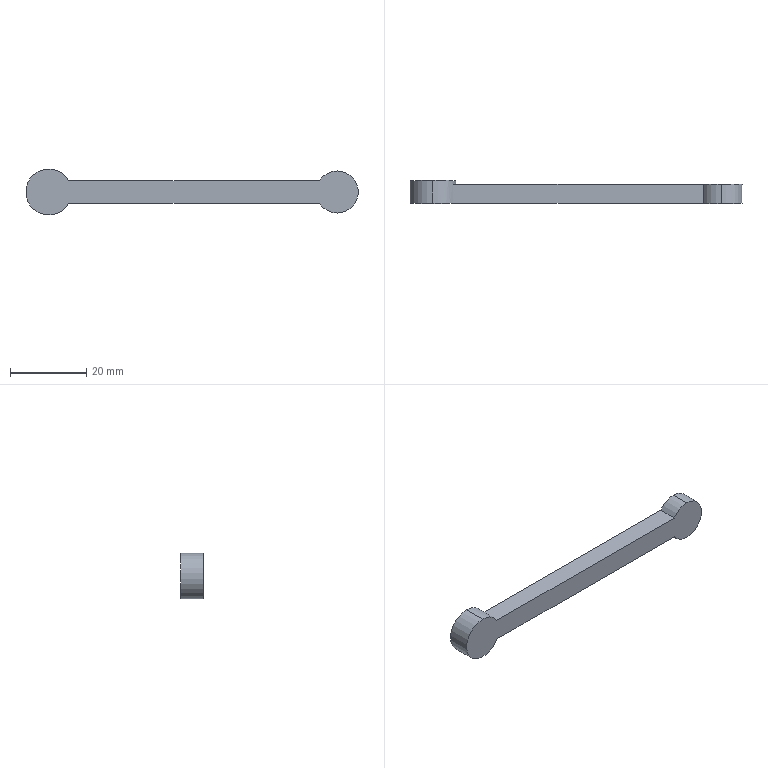Part | STEP file | 222_Default | 1 solid | 10 faces | box 86.9 x 6 x 12 mm | volume 3087 mm3 | cylinder 5 | plane 5 | commonest cylinder face diameters 11 x3 12 x2
STEP:
#1=CARTESIAN_POINT('',(0.,0.,0.));
#2=DIRECTION('',(0.,0.,1.));
#3=DIRECTION('',(1.,0.,0.));
#4=AXIS2_PLACEMENT_3D('',#1,#2,#3);
#5=CARTESIAN_POINT('',(37.7,0.,5.5));
#6=VERTEX_POINT('',#5);
#7=CARTESIAN_POINT('',(37.7,0.,-5.5));
#8=VERTEX_POINT('',#7);
#9=CARTESIAN_POINT('',(37.7,0.,0.));
#10=DIRECTION('',(0.,1.,0.));
#11=DIRECTION('',(0.,0.,1.));
#12=AXIS2_PLACEMENT_3D('',#9,#10,#11);
#13=CIRCLE('',#12,5.5);
#14=CARTESIAN_POINT('',(37.7,0.,0.));
#15=DIRECTION('',(0.,1.,0.));
#16=DIRECTION('',(0.,0.,1.));
#17=AXIS2_PLACEMENT_3D('',#14,#15,#16);
#18=CYLINDRICAL_SURFACE('',#17,5.5);
#19=CARTESIAN_POINT('',(0.,0.));
#20=DIRECTION('',(1.,0.));
#21=VECTOR('',#20,1.);
#22=LINE('',#19,#21);
#23=(GEOMETRIC_REPRESENTATION_CONTEXT(2)PARAMETRIC_REPRESENTATION_CONTEXT()REPRESENTATION_CONTEXT('',''));
#24=DEFINITIONAL_REPRESENTATION('',(#22),#23);
#25=PCURVE('',#18,#24);
#26=CARTESIAN_POINT('',(37.7,0.,0.));
#27=DIRECTION('',(0.,1.,0.));
#28=DIRECTION('',(0.,0.,1.));
#29=AXIS2_PLACEMENT_3D('',#26,#27,#28);
#30=PLANE('',#29);
#31=CARTESIAN_POINT('',(0.,0.));
#32=DIRECTION('',(1.,0.));
#33=AXIS2_PLACEMENT_2D('',#31,#32);
#34=CIRCLE('',#33,5.5);
#35=(GEOMETRIC_REPRESENTATION_CONTEXT(2)PARAMETRIC_REPRESENTATION_CONTEXT()REPRESENTATION_CONTEXT('',''));
#36=DEFINITIONAL_REPRESENTATION('',(#34),#35);
#37=PCURVE('',#30,#36);
#38=SURFACE_CURVE('',#13,(#25,#37),.PCURVE_S1.);
#39=EDGE_CURVE('',#6,#8,#38,.T.);
#40=ORIENTED_EDGE('',*,*,#39,.T.);
#41=CARTESIAN_POINT('',(37.7,5.,-5.5));
#42=VERTEX_POINT('',#41);
#43=CARTESIAN_POINT('',(37.7,0.,-5.5));
#44=DIRECTION('',(0.,1.,0.));
#45=VECTOR('',#44,1.);
#46=LINE('',#43,#45);
#47=CARTESIAN_POINT('',(3.142,0.));
#48=DIRECTION('',(0.,1.));
#49=VECTOR('',#48,1.);
#50=LINE('',#47,#49);
#51=(GEOMETRIC_REPRESENTATION_CONTEXT(2)PARAMETRIC_REPRESENTATION_CONTEXT()REPRESENTATION_CONTEXT('',''));
#52=DEFINITIONAL_REPRESENTATION('',(#50),#51);
#53=PCURVE('',#18,#52);
#54=CARTESIAN_POINT('',(37.7,0.,0.));
#55=DIRECTION('',(0.,1.,0.));
#56=DIRECTION('',(0.,0.,1.));
#57=AXIS2_PLACEMENT_3D('',#54,#55,#56);
#58=CYLINDRICAL_SURFACE('',#57,5.5);
#59=CARTESIAN_POINT('',(3.142,0.));
#60=DIRECTION('',(0.,1.));
#61=VECTOR('',#60,1.);
#62=LINE('',#59,#61);
#63=(GEOMETRIC_REPRESENTATION_CONTEXT(2)PARAMETRIC_REPRESENTATION_CONTEXT()REPRESENTATION_CONTEXT('',''));
#64=DEFINITIONAL_REPRESENTATION('',(#62),#63);
#65=PCURVE('',#58,#64);
#66=SURFACE_CURVE('',#46,(#53,#65),.PCURVE_S1.);
#67=EDGE_CURVE('',#8,#42,#66,.T.);
#68=ORIENTED_EDGE('',*,*,#67,.T.);
#69=CARTESIAN_POINT('',(37.7,5.,5.5));
#70=VERTEX_POINT('',#69);
#71=CARTESIAN_POINT('',(37.7,5.,0.));
#72=DIRECTION('',(0.,1.,0.));
#73=DIRECTION('',(0.,0.,1.));
#74=AXIS2_PLACEMENT_3D('',#71,#72,#73);
#75=CIRCLE('',#74,5.5);
#76=CARTESIAN_POINT('',(0.,5.));
#77=DIRECTION('',(1.,0.));
#78=VECTOR('',#77,1.);
#79=LINE('',#76,#78);
#80=(GEOMETRIC_REPRESENTATION_CONTEXT(2)PARAMETRIC_REPRESENTATION_CONTEXT()REPRESENTATION_CONTEXT('',''));
#81=DEFINITIONAL_REPRESENTATION('',(#79),#80);
#82=PCURVE('',#18,#81);
#83=CARTESIAN_POINT('',(37.7,5.,0.));
#84=DIRECTION('',(0.,1.,0.));
#85=DIRECTION('',(0.,0.,1.));
#86=AXIS2_PLACEMENT_3D('',#83,#84,#85);
#87=PLANE('',#86);
#88=CARTESIAN_POINT('',(0.,0.));
#89=DIRECTION('',(1.,0.));
#90=AXIS2_PLACEMENT_2D('',#88,#89);
#91=CIRCLE('',#90,5.5);
#92=(GEOMETRIC_REPRESENTATION_CONTEXT(2)PARAMETRIC_REPRESENTATION_CONTEXT()REPRESENTATION_CONTEXT('',''));
#93=DEFINITIONAL_REPRESENTATION('',(#91),#92);
#94=PCURVE('',#87,#93);
#95=SURFACE_CURVE('',#75,(#82,#94),.PCURVE_S1.);
#96=EDGE_CURVE('',#70,#42,#95,.T.);
#97=ORIENTED_EDGE('',*,*,#96,.F.);
#98=CARTESIAN_POINT('',(37.7,0.,5.5));
#99=DIRECTION('',(0.,1.,0.));
#100=VECTOR('',#99,1.);
#101=LINE('',#98,#100);
#102=CARTESIAN_POINT('',(0.,0.));
#103=DIRECTION('',(0.,1.));
#104=VECTOR('',#103,1.);
#105=LINE('',#102,#104);
#106=(GEOMETRIC_REPRESENTATION_CONTEXT(2)PARAMETRIC_REPRESENTATION_CONTEXT()REPRESENTATION_CONTEXT('',''));
#107=DEFINITIONAL_REPRESENTATION('',(#105),#106);
#108=PCURVE('',#18,#107);
#109=CARTESIAN_POINT('',(37.7,0.,0.));
#110=DIRECTION('',(0.,1.,0.));
#111=DIRECTION('',(0.,0.,1.));
#112=AXIS2_PLACEMENT_3D('',#109,#110,#111);
#113=CYLINDRICAL_SURFACE('',#112,5.5);
#114=CARTESIAN_POINT('',(6.283,0.));
#115=DIRECTION('',(0.,1.));
#116=VECTOR('',#115,1.);
#117=LINE('',#114,#116);
#118=(GEOMETRIC_REPRESENTATION_CONTEXT(2)PARAMETRIC_REPRESENTATION_CONTEXT()REPRESENTATION_CONTEXT('',''));
#119=DEFINITIONAL_REPRESENTATION('',(#117),#118);
#120=PCURVE('',#113,#119);
#121=SURFACE_CURVE('',#101,(#108,#120),.PCURVE_S1.);
#122=EDGE_CURVE('',#6,#70,#121,.T.);
#123=ORIENTED_EDGE('',*,*,#122,.F.);
#124=EDGE_LOOP('',(#40,#68,#97,#123));
#125=FACE_BOUND('',#124,.T.);
#126=ADVANCED_FACE('',(#125),#18,.T.);
#127=CARTESIAN_POINT('',(33.09,0.,3.));
#128=VERTEX_POINT('',#127);
#129=CARTESIAN_POINT('',(37.7,0.,0.));
#130=DIRECTION('',(0.,1.,0.));
#131=DIRECTION('',(0.,0.,1.));
#132=AXIS2_PLACEMENT_3D('',#129,#130,#131);
#133=CIRCLE('',#132,5.5);
#134=CARTESIAN_POINT('',(0.,0.));
#135=DIRECTION('',(1.,0.));
#136=VECTOR('',#135,1.);
#137=LINE('',#134,#136);
#138=(GEOMETRIC_REPRESENTATION_CONTEXT(2)PARAMETRIC_REPRESENTATION_CONTEXT()REPRESENTATION_CONTEXT('',''));
#139=DEFINITIONAL_REPRESENTATION('',(#137),#138);
#140=PCURVE('',#113,#139);
#141=CARTESIAN_POINT('',(0.,0.));
#142=DIRECTION('',(1.,0.));
#143=AXIS2_PLACEMENT_2D('',#141,#142);
#144=CIRCLE('',#143,5.5);
#145=(GEOMETRIC_REPRESENTATION_CONTEXT(2)PARAMETRIC_REPRESENTATION_CONTEXT()REPRESENTATION_CONTEXT('',''));
#146=DEFINITIONAL_REPRESENTATION('',(#144),#145);
#147=PCURVE('',#30,#146);
#148=SURFACE_CURVE('',#133,(#140,#147),.PCURVE_S1.);
#149=EDGE_CURVE('',#128,#6,#148,.T.);
#150=ORIENTED_EDGE('',*,*,#149,.T.);
#151=ORIENTED_EDGE('',*,*,#122,.T.);
#152=CARTESIAN_POINT('',(33.09,5.,3.));
#153=VERTEX_POINT('',#152);
#154=CARTESIAN_POINT('',(37.7,5.,0.));
#155=DIRECTION('',(0.,1.,0.));
#156=DIRECTION('',(0.,0.,1.));
#157=AXIS2_PLACEMENT_3D('',#154,#155,#156);
#158=CIRCLE('',#157,5.5);
#159=CARTESIAN_POINT('',(0.,5.));
#160=DIRECTION('',(1.,0.));
#161=VECTOR('',#160,1.);
#162=LINE('',#159,#161);
#163=(GEOMETRIC_REPRESENTATION_CONTEXT(2)PARAMETRIC_REPRESENTATION_CONTEXT()REPRESENTATION_CONTEXT('',''));
#164=DEFINITIONAL_REPRESENTATION('',(#162),#163);
#165=PCURVE('',#113,#164);
#166=CARTESIAN_POINT('',(0.,0.));
#167=DIRECTION('',(1.,0.));
#168=AXIS2_PLACEMENT_2D('',#166,#167);
#169=CIRCLE('',#168,5.5);
#170=(GEOMETRIC_REPRESENTATION_CONTEXT(2)PARAMETRIC_REPRESENTATION_CONTEXT()REPRESENTATION_CONTEXT('',''));
#171=DEFINITIONAL_REPRESENTATION('',(#169),#170);
#172=PCURVE('',#87,#171);
#173=SURFACE_CURVE('',#158,(#165,#172),.PCURVE_S1.);
#174=EDGE_CURVE('',#153,#70,#173,.T.);
#175=ORIENTED_EDGE('',*,*,#174,.F.);
#176=CARTESIAN_POINT('',(33.09,0.,3.));
#177=DIRECTION('',(0.,1.,0.));
#178=VECTOR('',#177,1.);
#179=LINE('',#176,#178);
#180=CARTESIAN_POINT('',(5.289,0.));
#181=DIRECTION('',(0.,1.));
#182=VECTOR('',#181,1.);
#183=LINE('',#180,#182);
#184=(GEOMETRIC_REPRESENTATION_CONTEXT(2)PARAMETRIC_REPRESENTATION_CONTEXT()REPRESENTATION_CONTEXT('',''));
#185=DEFINITIONAL_REPRESENTATION('',(#183),#184);
#186=PCURVE('',#113,#185);
#187=CARTESIAN_POINT('',(-32.504,0.,3.));
#188=DIRECTION('',(0.,0.,1.));
#189=DIRECTION('',(1.,0.,0.));
#190=AXIS2_PLACEMENT_3D('',#187,#188,#189);
#191=PLANE('',#190);
#192=CARTESIAN_POINT('',(65.594,0.));
#193=DIRECTION('',(0.,1.));
#194=VECTOR('',#193,1.);
#195=LINE('',#192,#194);
#196=(GEOMETRIC_REPRESENTATION_CONTEXT(2)PARAMETRIC_REPRESENTATION_CONTEXT()REPRESENTATION_CONTEXT('',''));
#197=DEFINITIONAL_REPRESENTATION('',(#195),#196);
#198=PCURVE('',#191,#197);
#199=SURFACE_CURVE('',#179,(#186,#198),.PCURVE_S1.);
#200=EDGE_CURVE('',#128,#153,#199,.T.);
#201=ORIENTED_EDGE('',*,*,#200,.F.);
#202=EDGE_LOOP('',(#150,#151,#175,#201));
#203=FACE_BOUND('',#202,.T.);
#204=ADVANCED_FACE('',(#203),#113,.T.);
#205=CARTESIAN_POINT('',(-37.7,6.,6.));
#206=VERTEX_POINT('',#205);
#207=CARTESIAN_POINT('',(-37.7,6.,-6.));
#208=VERTEX_POINT('',#207);
#209=CARTESIAN_POINT('',(-37.7,6.,0.));
#210=DIRECTION('',(0.,1.,0.));
#211=DIRECTION('',(0.,0.,1.));
#212=AXIS2_PLACEMENT_3D('',#209,#210,#211);
#213=CIRCLE('',#212,6.);
#214=CARTESIAN_POINT('',(-37.7,5.,0.));
#215=DIRECTION('',(0.,-1.,0.));
#216=DIRECTION('',(0.,0.,-1.));
#217=AXIS2_PLACEMENT_3D('',#214,#215,#216);
#218=CYLINDRICAL_SURFACE('',#217,6.);
#219=CARTESIAN_POINT('',(3.142,-1.));
#220=DIRECTION('',(-1.,0.));
#221=VECTOR('',#220,1.);
#222=LINE('',#219,#221);
#223=(GEOMETRIC_REPRESENTATION_CONTEXT(2)PARAMETRIC_REPRESENTATION_CONTEXT()REPRESENTATION_CONTEXT('',''));
#224=DEFINITIONAL_REPRESENTATION('',(#222),#223);
#225=PCURVE('',#218,#224);
#226=CARTESIAN_POINT('',(-37.7,6.,0.));
#227=DIRECTION('',(0.,1.,0.));
#228=DIRECTION('',(0.,0.,1.));
#229=AXIS2_PLACEMENT_3D('',#226,#227,#228);
#230=PLANE('',#229);
#231=CARTESIAN_POINT('',(0.,0.));
#232=DIRECTION('',(1.,0.));
#233=AXIS2_PLACEMENT_2D('',#231,#232);
#234=CIRCLE('',#233,6.);
#235=(GEOMETRIC_REPRESENTATION_CONTEXT(2)PARAMETRIC_REPRESENTATION_CONTEXT()REPRESENTATION_CONTEXT('',''));
#236=DEFINITIONAL_REPRESENTATION('',(#234),#235);
#237=PCURVE('',#230,#236);
#238=SURFACE_CURVE('',#213,(#225,#237),.PCURVE_S1.);
#239=EDGE_CURVE('',#206,#208,#238,.T.);
#240=ORIENTED_EDGE('',*,*,#239,.F.);
#241=CARTESIAN_POINT('',(-37.7,0.,6.));
#242=VERTEX_POINT('',#241);
#243=CARTESIAN_POINT('',(-37.7,5.,6.));
#244=DIRECTION('',(0.,-1.,0.));
#245=VECTOR('',#244,1.);
#246=LINE('',#243,#245);
#247=CARTESIAN_POINT('',(3.142,0.));
#248=DIRECTION('',(0.,1.));
#249=VECTOR('',#248,1.);
#250=LINE('',#247,#249);
#251=(GEOMETRIC_REPRESENTATION_CONTEXT(2)PARAMETRIC_REPRESENTATION_CONTEXT()REPRESENTATION_CONTEXT('',''));
#252=DEFINITIONAL_REPRESENTATION('',(#250),#251);
#253=PCURVE('',#218,#252);
#254=CARTESIAN_POINT('',(-37.7,5.,0.));
#255=DIRECTION('',(0.,-1.,0.));
#256=DIRECTION('',(0.,0.,-1.));
#257=AXIS2_PLACEMENT_3D('',#254,#255,#256);
#258=CYLINDRICAL_SURFACE('',#257,6.);
#259=CARTESIAN_POINT('',(3.142,0.));
#260=DIRECTION('',(0.,1.));
#261=VECTOR('',#260,1.);
#262=LINE('',#259,#261);
#263=(GEOMETRIC_REPRESENTATION_CONTEXT(2)PARAMETRIC_REPRESENTATION_CONTEXT()REPRESENTATION_CONTEXT('',''));
#264=DEFINITIONAL_REPRESENTATION('',(#262),#263);
#265=PCURVE('',#258,#264);
#266=SURFACE_CURVE('',#246,(#253,#265),.PCURVE_S1.);
#267=EDGE_CURVE('',#206,#242,#266,.T.);
#268=ORIENTED_EDGE('',*,*,#267,.T.);
#269=CARTESIAN_POINT('',(-32.504,0.,3.));
#270=VERTEX_POINT('',#269);
#271=CARTESIAN_POINT('',(-37.7,0.,0.));
#272=DIRECTION('',(0.,1.,0.));
#273=DIRECTION('',(0.,0.,1.));
#274=AXIS2_PLACEMENT_3D('',#271,#272,#273);
#275=CIRCLE('',#274,6.);
#276=CARTESIAN_POINT('',(3.142,5.));
#277=DIRECTION('',(-1.,0.));
#278=VECTOR('',#277,1.);
#279=LINE('',#276,#278);
#280=(GEOMETRIC_REPRESENTATION_CONTEXT(2)PARAMETRIC_REPRESENTATION_CONTEXT()REPRESENTATION_CONTEXT('',''));
#281=DEFINITIONAL_REPRESENTATION('',(#279),#280);
#282=PCURVE('',#218,#281);
#283=CARTESIAN_POINT('',(0.,-75.4));
#284=DIRECTION('',(1.,0.));
#285=AXIS2_PLACEMENT_2D('',#283,#284);
#286=CIRCLE('',#285,6.);
#287=(GEOMETRIC_REPRESENTATION_CONTEXT(2)PARAMETRIC_REPRESENTATION_CONTEXT()REPRESENTATION_CONTEXT('',''));
#288=DEFINITIONAL_REPRESENTATION('',(#286),#287);
#289=PCURVE('',#30,#288);
#290=SURFACE_CURVE('',#275,(#282,#289),.PCURVE_S1.);
#291=EDGE_CURVE('',#242,#270,#290,.T.);
#292=ORIENTED_EDGE('',*,*,#291,.T.);
#293=CARTESIAN_POINT('',(-32.504,5.,3.));
#294=VERTEX_POINT('',#293);
#295=CARTESIAN_POINT('',(-32.504,0.,3.));
#296=DIRECTION('',(0.,1.,0.));
#297=VECTOR('',#296,1.);
#298=LINE('',#295,#297);
#299=CARTESIAN_POINT('',(2.094,5.));
#300=DIRECTION('',(0.,-1.));
#301=VECTOR('',#300,1.);
#302=LINE('',#299,#301);
#303=(GEOMETRIC_REPRESENTATION_CONTEXT(2)PARAMETRIC_REPRESENTATION_CONTEXT()REPRESENTATION_CONTEXT('',''));
#304=DEFINITIONAL_REPRESENTATION('',(#302),#303);
#305=PCURVE('',#218,#304);
#306=CARTESIAN_POINT('',(0.,0.));
#307=DIRECTION('',(0.,1.));
#308=VECTOR('',#307,1.);
#309=LINE('',#306,#308);
#310=(GEOMETRIC_REPRESENTATION_CONTEXT(2)PARAMETRIC_REPRESENTATION_CONTEXT()REPRESENTATION_CONTEXT('',''));
#311=DEFINITIONAL_REPRESENTATION('',(#309),#310);
#312=PCURVE('',#191,#311);
#313=SURFACE_CURVE('',#298,(#305,#312),.PCURVE_S1.);
#314=EDGE_CURVE('',#270,#294,#313,.T.);
#315=ORIENTED_EDGE('',*,*,#314,.T.);
#316=CARTESIAN_POINT('',(-32.504,5.,-3.));
#317=VERTEX_POINT('',#316);
#318=CARTESIAN_POINT('',(-37.7,5.,0.));
#319=DIRECTION('',(0.,1.,0.));
#320=DIRECTION('',(0.,0.,1.));
#321=AXIS2_PLACEMENT_3D('',#318,#319,#320);
#322=CIRCLE('',#321,6.);
#323=CARTESIAN_POINT('',(3.142,0.));
#324=DIRECTION('',(-1.,0.));
#325=VECTOR('',#324,1.);
#326=LINE('',#323,#325);
#327=(GEOMETRIC_REPRESENTATION_CONTEXT(2)PARAMETRIC_REPRESENTATION_CONTEXT()REPRESENTATION_CONTEXT('',''));
#328=DEFINITIONAL_REPRESENTATION('',(#326),#327);
#329=PCURVE('',#218,#328);
#330=CARTESIAN_POINT('',(0.,-75.4));
#331=DIRECTION('',(1.,0.));
#332=AXIS2_PLACEMENT_2D('',#330,#331);
#333=CIRCLE('',#332,6.);
#334=(GEOMETRIC_REPRESENTATION_CONTEXT(2)PARAMETRIC_REPRESENTATION_CONTEXT()REPRESENTATION_CONTEXT('',''));
#335=DEFINITIONAL_REPRESENTATION('',(#333),#334);
#336=PCURVE('',#87,#335);
#337=SURFACE_CURVE('',#322,(#329,#336),.PCURVE_S1.);
#338=EDGE_CURVE('',#294,#317,#337,.T.);
#339=ORIENTED_EDGE('',*,*,#338,.T.);
#340=CARTESIAN_POINT('',(-32.504,0.,-3.));
#341=VERTEX_POINT('',#340);
#342=CARTESIAN_POINT('',(-32.504,0.,-3.));
#343=DIRECTION('',(0.,1.,0.));
#344=VECTOR('',#343,1.);
#345=LINE('',#342,#344);
#346=CARTESIAN_POINT('',(1.047,5.));
#347=DIRECTION('',(0.,-1.));
#348=VECTOR('',#347,1.);
#349=LINE('',#346,#348);
#350=(GEOMETRIC_REPRESENTATION_CONTEXT(2)PARAMETRIC_REPRESENTATION_CONTEXT()REPRESENTATION_CONTEXT('',''));
#351=DEFINITIONAL_REPRESENTATION('',(#349),#350);
#352=PCURVE('',#218,#351);
#353=CARTESIAN_POINT('',(-32.504,0.,-3.));
#354=DIRECTION('',(0.,0.,-1.));
#355=DIRECTION('',(-1.,0.,0.));
#356=AXIS2_PLACEMENT_3D('',#353,#354,#355);
#357=PLANE('',#356);
#358=CARTESIAN_POINT('',(0.,0.));
#359=DIRECTION('',(0.,1.));
#360=VECTOR('',#359,1.);
#361=LINE('',#358,#360);
#362=(GEOMETRIC_REPRESENTATION_CONTEXT(2)PARAMETRIC_REPRESENTATION_CONTEXT()REPRESENTATION_CONTEXT('',''));
#363=DEFINITIONAL_REPRESENTATION('',(#361),#362);
#364=PCURVE('',#357,#363);
#365=SURFACE_CURVE('',#345,(#352,#364),.PCURVE_S1.);
#366=EDGE_CURVE('',#341,#317,#365,.T.);
#367=ORIENTED_EDGE('',*,*,#366,.F.);
#368=CARTESIAN_POINT('',(-37.7,0.,-6.));
#369=VERTEX_POINT('',#368);
#370=CARTESIAN_POINT('',(-37.7,0.,0.));
#371=DIRECTION('',(0.,1.,0.));
#372=DIRECTION('',(0.,0.,1.));
#373=AXIS2_PLACEMENT_3D('',#370,#371,#372);
#374=CIRCLE('',#373,6.);
#375=CARTESIAN_POINT('',(3.142,5.));
#376=DIRECTION('',(-1.,0.));
#377=VECTOR('',#376,1.);
#378=LINE('',#375,#377);
#379=(GEOMETRIC_REPRESENTATION_CONTEXT(2)PARAMETRIC_REPRESENTATION_CONTEXT()REPRESENTATION_CONTEXT('',''));
#380=DEFINITIONAL_REPRESENTATION('',(#378),#379);
#381=PCURVE('',#218,#380);
#382=CARTESIAN_POINT('',(0.,-75.4));
#383=DIRECTION('',(1.,0.));
#384=AXIS2_PLACEMENT_2D('',#382,#383);
#385=CIRCLE('',#384,6.);
#386=(GEOMETRIC_REPRESENTATION_CONTEXT(2)PARAMETRIC_REPRESENTATION_CONTEXT()REPRESENTATION_CONTEXT('',''));
#387=DEFINITIONAL_REPRESENTATION('',(#385),#386);
#388=PCURVE('',#30,#387);
#389=SURFACE_CURVE('',#374,(#381,#388),.PCURVE_S1.);
#390=EDGE_CURVE('',#341,#369,#389,.T.);
#391=ORIENTED_EDGE('',*,*,#390,.T.);
#392=CARTESIAN_POINT('',(-37.7,5.,-6.));
#393=DIRECTION('',(0.,-1.,0.));
#394=VECTOR('',#393,1.);
#395=LINE('',#392,#394);
#396=CARTESIAN_POINT('',(0.,0.));
#397=DIRECTION('',(0.,1.));
#398=VECTOR('',#397,1.);
#399=LINE('',#396,#398);
#400=(GEOMETRIC_REPRESENTATION_CONTEXT(2)PARAMETRIC_REPRESENTATION_CONTEXT()REPRESENTATION_CONTEXT('',''));
#401=DEFINITIONAL_REPRESENTATION('',(#399),#400);
#402=PCURVE('',#218,#401);
#403=CARTESIAN_POINT('',(6.283,0.));
#404=DIRECTION('',(0.,1.));
#405=VECTOR('',#404,1.);
#406=LINE('',#403,#405);
#407=(GEOMETRIC_REPRESENTATION_CONTEXT(2)PARAMETRIC_REPRESENTATION_CONTEXT()REPRESENTATION_CONTEXT('',''));
#408=DEFINITIONAL_REPRESENTATION('',(#406),#407);
#409=PCURVE('',#258,#408);
#410=SURFACE_CURVE('',#395,(#402,#409),.PCURVE_S1.);
#411=EDGE_CURVE('',#208,#369,#410,.T.);
#412=ORIENTED_EDGE('',*,*,#411,.F.);
#413=EDGE_LOOP('',(#240,#268,#292,#315,#339,#367,#391,#412));
#414=FACE_BOUND('',#413,.T.);
#415=ADVANCED_FACE('',(#414),#218,.T.);
#416=ORIENTED_EDGE('',*,*,#338,.F.);
#417=CARTESIAN_POINT('',(-32.504,5.,3.));
#418=DIRECTION('',(1.,0.,0.));
#419=VECTOR('',#418,1.);
#420=LINE('',#417,#419);
#421=CARTESIAN_POINT('',(3.,-70.204));
#422=DIRECTION('',(0.,1.));
#423=VECTOR('',#422,1.);
#424=LINE('',#421,#423);
#425=(GEOMETRIC_REPRESENTATION_CONTEXT(2)PARAMETRIC_REPRESENTATION_CONTEXT()REPRESENTATION_CONTEXT('',''));
#426=DEFINITIONAL_REPRESENTATION('',(#424),#425);
#427=PCURVE('',#87,#426);
#428=CARTESIAN_POINT('',(0.,5.));
#429=DIRECTION('',(1.,0.));
#430=VECTOR('',#429,1.);
#431=LINE('',#428,#430);
#432=(GEOMETRIC_REPRESENTATION_CONTEXT(2)PARAMETRIC_REPRESENTATION_CONTEXT()REPRESENTATION_CONTEXT('',''));
#433=DEFINITIONAL_REPRESENTATION('',(#431),#432);
#434=PCURVE('',#191,#433);
#435=SURFACE_CURVE('',#420,(#427,#434),.PCURVE_S1.);
#436=EDGE_CURVE('',#294,#153,#435,.T.);
#437=ORIENTED_EDGE('',*,*,#436,.T.);
#438=ORIENTED_EDGE('',*,*,#174,.T.);
#439=ORIENTED_EDGE('',*,*,#96,.T.);
#440=CARTESIAN_POINT('',(33.09,5.,-3.));
#441=VERTEX_POINT('',#440);
#442=CARTESIAN_POINT('',(37.7,5.,0.));
#443=DIRECTION('',(0.,1.,0.));
#444=DIRECTION('',(0.,0.,1.));
#445=AXIS2_PLACEMENT_3D('',#442,#443,#444);
#446=CIRCLE('',#445,5.5);
#447=CARTESIAN_POINT('',(0.,0.));
#448=DIRECTION('',(1.,0.));
#449=AXIS2_PLACEMENT_2D('',#447,#448);
#450=CIRCLE('',#449,5.5);
#451=(GEOMETRIC_REPRESENTATION_CONTEXT(2)PARAMETRIC_REPRESENTATION_CONTEXT()REPRESENTATION_CONTEXT('',''));
#452=DEFINITIONAL_REPRESENTATION('',(#450),#451);
#453=PCURVE('',#87,#452);
#454=CARTESIAN_POINT('',(0.,5.));
#455=DIRECTION('',(1.,0.));
#456=VECTOR('',#455,1.);
#457=LINE('',#454,#456);
#458=(GEOMETRIC_REPRESENTATION_CONTEXT(2)PARAMETRIC_REPRESENTATION_CONTEXT()REPRESENTATION_CONTEXT('',''));
#459=DEFINITIONAL_REPRESENTATION('',(#457),#458);
#460=PCURVE('',#58,#459);
#461=SURFACE_CURVE('',#446,(#453,#460),.PCURVE_S1.);
#462=EDGE_CURVE('',#42,#441,#461,.T.);
#463=ORIENTED_EDGE('',*,*,#462,.T.);
#464=CARTESIAN_POINT('',(-32.504,5.,-3.));
#465=DIRECTION('',(-1.,0.,0.));
#466=VECTOR('',#465,1.);
#467=LINE('',#464,#466);
#468=CARTESIAN_POINT('',(-3.,-70.204));
#469=DIRECTION('',(0.,-1.));
#470=VECTOR('',#469,1.);
#471=LINE('',#468,#470);
#472=(GEOMETRIC_REPRESENTATION_CONTEXT(2)PARAMETRIC_REPRESENTATION_CONTEXT()REPRESENTATION_CONTEXT('',''));
#473=DEFINITIONAL_REPRESENTATION('',(#471),#472);
#474=PCURVE('',#87,#473);
#475=CARTESIAN_POINT('',(0.,5.));
#476=DIRECTION('',(1.,0.));
#477=VECTOR('',#476,1.);
#478=LINE('',#475,#477);
#479=(GEOMETRIC_REPRESENTATION_CONTEXT(2)PARAMETRIC_REPRESENTATION_CONTEXT()REPRESENTATION_CONTEXT('',''));
#480=DEFINITIONAL_REPRESENTATION('',(#478),#479);
#481=PCURVE('',#357,#480);
#482=SURFACE_CURVE('',#467,(#474,#481),.PCURVE_S1.);
#483=EDGE_CURVE('',#441,#317,#482,.T.);
#484=ORIENTED_EDGE('',*,*,#483,.T.);
#485=EDGE_LOOP('',(#416,#437,#438,#439,#463,#484));
#486=FACE_BOUND('',#485,.T.);
#487=ADVANCED_FACE('',(#486),#87,.T.);
#488=CARTESIAN_POINT('',(-32.504,0.,3.));
#489=DIRECTION('',(1.,0.,0.));
#490=VECTOR('',#489,1.);
#491=LINE('',#488,#490);
#492=CARTESIAN_POINT('',(3.,-70.204));
#493=DIRECTION('',(0.,1.));
#494=VECTOR('',#493,1.);
#495=LINE('',#492,#494);
#496=(GEOMETRIC_REPRESENTATION_CONTEXT(2)PARAMETRIC_REPRESENTATION_CONTEXT()REPRESENTATION_CONTEXT('',''));
#497=DEFINITIONAL_REPRESENTATION('',(#495),#496);
#498=PCURVE('',#30,#497);
#499=CARTESIAN_POINT('',(0.,0.));
#500=DIRECTION('',(1.,0.));
#501=VECTOR('',#500,1.);
#502=LINE('',#499,#501);
#503=(GEOMETRIC_REPRESENTATION_CONTEXT(2)PARAMETRIC_REPRESENTATION_CONTEXT()REPRESENTATION_CONTEXT('',''));
#504=DEFINITIONAL_REPRESENTATION('',(#502),#503);
#505=PCURVE('',#191,#504);
#506=SURFACE_CURVE('',#491,(#498,#505),.PCURVE_S1.);
#507=EDGE_CURVE('',#270,#128,#506,.T.);
#508=ORIENTED_EDGE('',*,*,#507,.F.);
#509=ORIENTED_EDGE('',*,*,#291,.F.);
#510=CARTESIAN_POINT('',(-37.7,0.,0.));
#511=DIRECTION('',(0.,1.,0.));
#512=DIRECTION('',(0.,0.,1.));
#513=AXIS2_PLACEMENT_3D('',#510,#511,#512);
#514=CIRCLE('',#513,6.);
#515=CARTESIAN_POINT('',(0.,-75.4));
#516=DIRECTION('',(1.,0.));
#517=AXIS2_PLACEMENT_2D('',#515,#516);
#518=CIRCLE('',#517,6.);
#519=(GEOMETRIC_REPRESENTATION_CONTEXT(2)PARAMETRIC_REPRESENTATION_CONTEXT()REPRESENTATION_CONTEXT('',''));
#520=DEFINITIONAL_REPRESENTATION('',(#518),#519);
#521=PCURVE('',#30,#520);
#522=CARTESIAN_POINT('',(9.425,5.));
#523=DIRECTION('',(-1.,0.));
#524=VECTOR('',#523,1.);
#525=LINE('',#522,#524);
#526=(GEOMETRIC_REPRESENTATION_CONTEXT(2)PARAMETRIC_REPRESENTATION_CONTEXT()REPRESENTATION_CONTEXT('',''));
#527=DEFINITIONAL_REPRESENTATION('',(#525),#526);
#528=PCURVE('',#258,#527);
#529=SURFACE_CURVE('',#514,(#521,#528),.PCURVE_S1.);
#530=EDGE_CURVE('',#369,#242,#529,.T.);
#531=ORIENTED_EDGE('',*,*,#530,.F.);
#532=ORIENTED_EDGE('',*,*,#390,.F.);
#533=CARTESIAN_POINT('',(33.09,0.,-3.));
#534=VERTEX_POINT('',#533);
#535=CARTESIAN_POINT('',(-32.504,0.,-3.));
#536=DIRECTION('',(-1.,0.,0.));
#537=VECTOR('',#536,1.);
#538=LINE('',#535,#537);
#539=CARTESIAN_POINT('',(-3.,-70.204));
#540=DIRECTION('',(0.,-1.));
#541=VECTOR('',#540,1.);
#542=LINE('',#539,#541);
#543=(GEOMETRIC_REPRESENTATION_CONTEXT(2)PARAMETRIC_REPRESENTATION_CONTEXT()REPRESENTATION_CONTEXT('',''));
#544=DEFINITIONAL_REPRESENTATION('',(#542),#543);
#545=PCURVE('',#30,#544);
#546=CARTESIAN_POINT('',(0.,0.));
#547=DIRECTION('',(1.,0.));
#548=VECTOR('',#547,1.);
#549=LINE('',#546,#548);
#550=(GEOMETRIC_REPRESENTATION_CONTEXT(2)PARAMETRIC_REPRESENTATION_CONTEXT()REPRESENTATION_CONTEXT('',''));
#551=DEFINITIONAL_REPRESENTATION('',(#549),#550);
#552=PCURVE('',#357,#551);
#553=SURFACE_CURVE('',#538,(#545,#552),.PCURVE_S1.);
#554=EDGE_CURVE('',#534,#341,#553,.T.);
#555=ORIENTED_EDGE('',*,*,#554,.F.);
#556=CARTESIAN_POINT('',(37.7,0.,0.));
#557=DIRECTION('',(0.,1.,0.));
#558=DIRECTION('',(0.,0.,1.));
#559=AXIS2_PLACEMENT_3D('',#556,#557,#558);
#560=CIRCLE('',#559,5.5);
#561=CARTESIAN_POINT('',(0.,0.));
#562=DIRECTION('',(1.,0.));
#563=AXIS2_PLACEMENT_2D('',#561,#562);
#564=CIRCLE('',#563,5.5);
#565=(GEOMETRIC_REPRESENTATION_CONTEXT(2)PARAMETRIC_REPRESENTATION_CONTEXT()REPRESENTATION_CONTEXT('',''));
#566=DEFINITIONAL_REPRESENTATION('',(#564),#565);
#567=PCURVE('',#30,#566);
#568=CARTESIAN_POINT('',(0.,0.));
#569=DIRECTION('',(1.,0.));
#570=VECTOR('',#569,1.);
#571=LINE('',#568,#570);
#572=(GEOMETRIC_REPRESENTATION_CONTEXT(2)PARAMETRIC_REPRESENTATION_CONTEXT()REPRESENTATION_CONTEXT('',''));
#573=DEFINITIONAL_REPRESENTATION('',(#571),#572);
#574=PCURVE('',#58,#573);
#575=SURFACE_CURVE('',#560,(#567,#574),.PCURVE_S1.);
#576=EDGE_CURVE('',#8,#534,#575,.T.);
#577=ORIENTED_EDGE('',*,*,#576,.F.);
#578=ORIENTED_EDGE('',*,*,#39,.F.);
#579=ORIENTED_EDGE('',*,*,#149,.F.);
#580=EDGE_LOOP('',(#508,#509,#531,#532,#555,#577,#578,#579));
#581=FACE_BOUND('',#580,.T.);
#582=ADVANCED_FACE('',(#581),#30,.F.);
#583=ORIENTED_EDGE('',*,*,#267,.F.);
#584=CARTESIAN_POINT('',(-37.7,6.,0.));
#585=DIRECTION('',(0.,1.,0.));
#586=DIRECTION('',(0.,0.,1.));
#587=AXIS2_PLACEMENT_3D('',#584,#585,#586);
#588=CIRCLE('',#587,6.);
#589=CARTESIAN_POINT('',(9.425,-1.));
#590=DIRECTION('',(-1.,0.));
#591=VECTOR('',#590,1.);
#592=LINE('',#589,#591);
#593=(GEOMETRIC_REPRESENTATION_CONTEXT(2)PARAMETRIC_REPRESENTATION_CONTEXT()REPRESENTATION_CONTEXT('',''));
#594=DEFINITIONAL_REPRESENTATION('',(#592),#593);
#595=PCURVE('',#258,#594);
#596=CARTESIAN_POINT('',(0.,0.));
#597=DIRECTION('',(1.,0.));
#598=AXIS2_PLACEMENT_2D('',#596,#597);
#599=CIRCLE('',#598,6.);
#600=(GEOMETRIC_REPRESENTATION_CONTEXT(2)PARAMETRIC_REPRESENTATION_CONTEXT()REPRESENTATION_CONTEXT('',''));
#601=DEFINITIONAL_REPRESENTATION('',(#599),#600);
#602=PCURVE('',#230,#601);
#603=SURFACE_CURVE('',#588,(#595,#602),.PCURVE_S1.);
#604=EDGE_CURVE('',#208,#206,#603,.T.);
#605=ORIENTED_EDGE('',*,*,#604,.F.);
#606=ORIENTED_EDGE('',*,*,#411,.T.);
#607=ORIENTED_EDGE('',*,*,#530,.T.);
#608=EDGE_LOOP('',(#583,#605,#606,#607));
#609=FACE_BOUND('',#608,.T.);
#610=ADVANCED_FACE('',(#609),#258,.T.);
#611=ORIENTED_EDGE('',*,*,#67,.F.);
#612=ORIENTED_EDGE('',*,*,#576,.T.);
#613=CARTESIAN_POINT('',(33.09,0.,-3.));
#614=DIRECTION('',(0.,1.,0.));
#615=VECTOR('',#614,1.);
#616=LINE('',#613,#615);
#617=CARTESIAN_POINT('',(4.135,0.));
#618=DIRECTION('',(0.,1.));
#619=VECTOR('',#618,1.);
#620=LINE('',#617,#619);
#621=(GEOMETRIC_REPRESENTATION_CONTEXT(2)PARAMETRIC_REPRESENTATION_CONTEXT()REPRESENTATION_CONTEXT('',''));
#622=DEFINITIONAL_REPRESENTATION('',(#620),#621);
#623=PCURVE('',#58,#622);
#624=CARTESIAN_POINT('',(-65.594,0.));
#625=DIRECTION('',(0.,1.));
#626=VECTOR('',#625,1.);
#627=LINE('',#624,#626);
#628=(GEOMETRIC_REPRESENTATION_CONTEXT(2)PARAMETRIC_REPRESENTATION_CONTEXT()REPRESENTATION_CONTEXT('',''));
#629=DEFINITIONAL_REPRESENTATION('',(#627),#628);
#630=PCURVE('',#357,#629);
#631=SURFACE_CURVE('',#616,(#623,#630),.PCURVE_S1.);
#632=EDGE_CURVE('',#534,#441,#631,.T.);
#633=ORIENTED_EDGE('',*,*,#632,.T.);
#634=ORIENTED_EDGE('',*,*,#462,.F.);
#635=EDGE_LOOP('',(#611,#612,#633,#634));
#636=FACE_BOUND('',#635,.T.);
#637=ADVANCED_FACE('',(#636),#58,.T.);
#638=ORIENTED_EDGE('',*,*,#436,.F.);
#639=ORIENTED_EDGE('',*,*,#314,.F.);
#640=ORIENTED_EDGE('',*,*,#507,.T.);
#641=ORIENTED_EDGE('',*,*,#200,.T.);
#642=EDGE_LOOP('',(#638,#639,#640,#641));
#643=FACE_BOUND('',#642,.T.);
#644=ADVANCED_FACE('',(#643),#191,.T.);
#645=ORIENTED_EDGE('',*,*,#483,.F.);
#646=ORIENTED_EDGE('',*,*,#632,.F.);
#647=ORIENTED_EDGE('',*,*,#554,.T.);
#648=ORIENTED_EDGE('',*,*,#366,.T.);
#649=EDGE_LOOP('',(#645,#646,#647,#648));
#650=FACE_BOUND('',#649,.T.);
#651=ADVANCED_FACE('',(#650),#357,.T.);
#652=ORIENTED_EDGE('',*,*,#604,.T.);
#653=ORIENTED_EDGE('',*,*,#239,.T.);
#654=EDGE_LOOP('',(#652,#653));
#655=FACE_BOUND('',#654,.T.);
#656=ADVANCED_FACE('',(#655),#230,.T.);
#657=CLOSED_SHELL('',(#126,#204,#415,#487,#582,#610,#637,#644,#651,#656));
#658=MANIFOLD_SOLID_BREP('',#657);
#659=(LENGTH_UNIT()NAMED_UNIT(*)SI_UNIT(.MILLI.,.METRE.));
#660=UNCERTAINTY_MEASURE_WITH_UNIT(LENGTH_MEASURE(0.0000001),#659,'','');
#661=(NAMED_UNIT(*)PLANE_ANGLE_UNIT()SI_UNIT($,.RADIAN.));
#662=(NAMED_UNIT(*)SI_UNIT($,.STERADIAN.)SOLID_ANGLE_UNIT());
#663=(GEOMETRIC_REPRESENTATION_CONTEXT(3)GLOBAL_UNCERTAINTY_ASSIGNED_CONTEXT((#660))GLOBAL_UNIT_ASSIGNED_CONTEXT((#659,#661,#662))REPRESENTATION_CONTEXT('',''));
#664=ADVANCED_BREP_SHAPE_REPRESENTATION('',(#4,#658),#663);